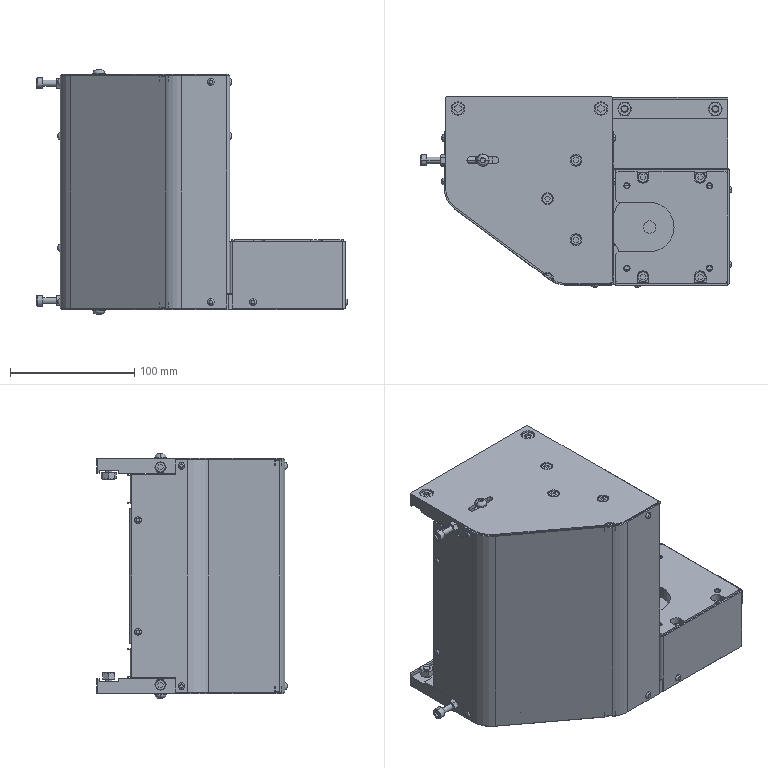Part | STEP file | Guide wheel mechanism revised.sldasm-Part-75 | 1 solid | 1023 faces | box 249.85 x 152.85 x 196.5 mm | volume 1149305 mm3 | plane 574 | cylinder 275 | cone 146 | torus 28 | commonest cylinder face diameters 8.5 x36 9.5 x28 10 x24 7 x16 7.6 x16 54 x16